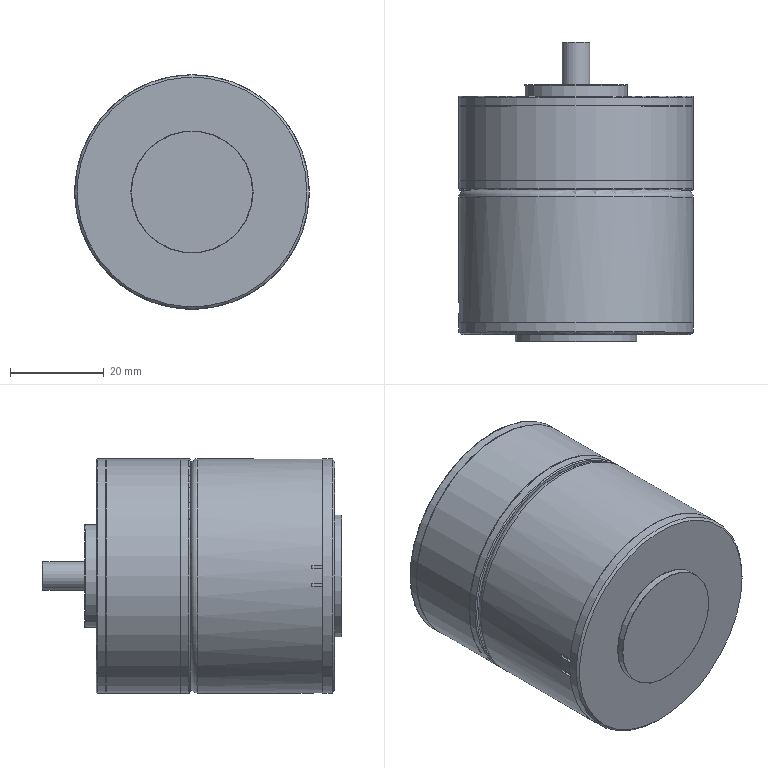Part | STEP file | zhiliudianji_Ratio 171 & 226 | 7 solids | 79 faces | box 50 x 63.8 x 50 mm | volume 24472 mm3 | plane 40 | cylinder 28 | torus 7 | cone 4 | commonest cylinder face diameters 0.8 x8 50 x5 1.5 x2 4 x2 49 x2 6 x1